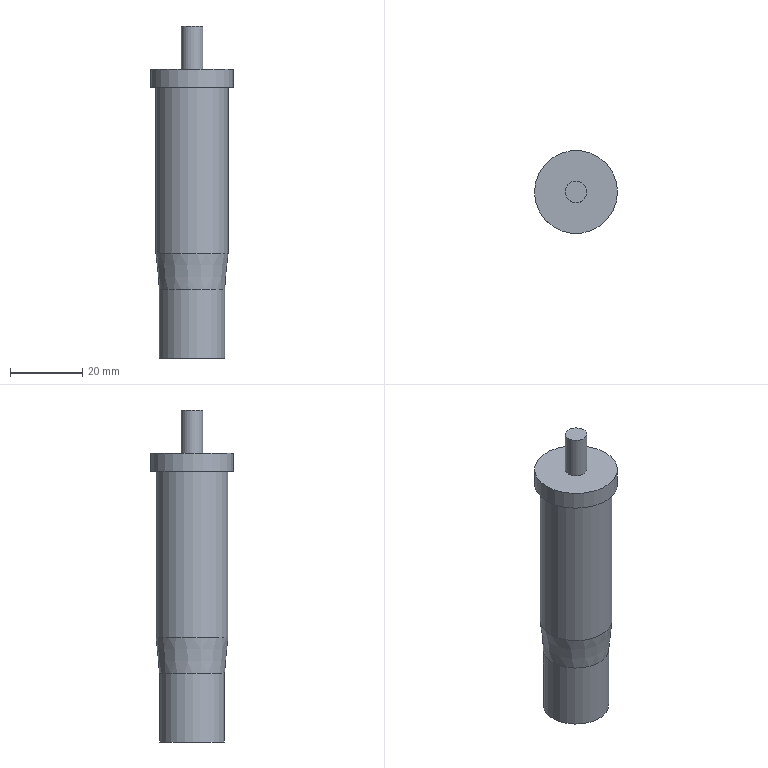Part | NX | features solid 2 | 1 solid | 9 faces | box 23 x 23 x 92 mm | volume 24609 mm3 | plane 4 | cylinder 4 | cone 1 | commonest cylinder face diameters 6 x1 18.1 x1 20 x1 23 x1
STEP:
#1=CARTESIAN_POINT('',(495.412,-159.012,39.));
#2=VERTEX_POINT('',#1);
#3=CARTESIAN_POINT('',(486.67,-161.354,39.));
#4=DIRECTION('',(0.,0.,1.));
#5=DIRECTION('',(0.9659,0.2588,0.));
#6=AXIS2_PLACEMENT_3D('',#3,#4,#5);
#7=CIRCLE('',#6,9.05);
#8=EDGE_CURVE('',#2,#2,#7,.T.);
#9=ORIENTED_EDGE('',*,*,#8,.F.);
#10=EDGE_LOOP('',(#9));
#11=FACE_BOUND('',#10,.T.);
#12=CARTESIAN_POINT('',(486.67,-161.354,39.));
#13=DIRECTION('',(0.,0.,-1.));
#14=DIRECTION('',(-0.9659,-0.2588,0.));
#15=AXIS2_PLACEMENT_3D('',#12,#13,#14);
#16=PLANE('',#15);
#17=ADVANCED_FACE('',(#11),#16,.T.);
#18=CARTESIAN_POINT('',(495.412,-159.012,58.));
#19=VERTEX_POINT('',#18);
#20=CARTESIAN_POINT('',(486.67,-161.354,58.));
#21=DIRECTION('',(0.,0.,1.));
#22=DIRECTION('',(0.9659,0.2588,0.));
#23=AXIS2_PLACEMENT_3D('',#20,#21,#22);
#24=CIRCLE('',#23,9.05);
#25=EDGE_CURVE('',#19,#19,#24,.T.);
#26=ORIENTED_EDGE('',*,*,#25,.F.);
#27=EDGE_LOOP('',(#26));
#28=FACE_BOUND('',#27,.T.);
#29=ORIENTED_EDGE('',*,*,#8,.T.);
#30=EDGE_LOOP('',(#29));
#31=FACE_BOUND('',#30,.T.);
#32=CARTESIAN_POINT('',(486.67,-161.354,39.));
#33=DIRECTION('',(0.,0.,1.));
#34=DIRECTION('',(0.9659,0.2588,0.));
#35=AXIS2_PLACEMENT_3D('',#32,#33,#34);
#36=CYLINDRICAL_SURFACE('',#35,9.05);
#37=ADVANCED_FACE('',(#28,#31),#36,.T.);
#38=ORIENTED_EDGE('',*,*,#25,.T.);
#39=EDGE_LOOP('',(#38));
#40=FACE_BOUND('',#39,.T.);
#41=CARTESIAN_POINT('',(496.329,-158.766,68.));
#42=VERTEX_POINT('',#41);
#43=CARTESIAN_POINT('',(486.67,-161.354,68.));
#44=DIRECTION('',(0.,0.,1.));
#45=DIRECTION('',(0.9659,0.2588,0.));
#46=AXIS2_PLACEMENT_3D('',#43,#44,#45);
#47=CIRCLE('',#46,10.);
#48=EDGE_CURVE('',#42,#42,#47,.T.);
#49=ORIENTED_EDGE('',*,*,#48,.F.);
#50=EDGE_LOOP('',(#49));
#51=FACE_BOUND('',#50,.T.);
#52=CARTESIAN_POINT('',(486.67,-161.354,58.));
#53=DIRECTION('',(0.,0.,1.));
#54=DIRECTION('',(0.9659,0.2588,0.));
#55=AXIS2_PLACEMENT_3D('',#52,#53,#54);
#56=CONICAL_SURFACE('',#55,9.05,0.09472);
#57=ADVANCED_FACE('',(#40,#51),#56,.T.);
#58=CARTESIAN_POINT('',(477.011,-163.943,114.));
#59=VERTEX_POINT('',#58);
#60=CARTESIAN_POINT('',(486.67,-161.354,114.));
#61=DIRECTION('',(0.,0.,-1.));
#62=DIRECTION('',(-0.9659,-0.2588,0.));
#63=AXIS2_PLACEMENT_3D('',#60,#61,#62);
#64=CIRCLE('',#63,10.);
#65=EDGE_CURVE('',#59,#59,#64,.F.);
#66=ORIENTED_EDGE('',*,*,#65,.F.);
#67=EDGE_LOOP('',(#66));
#68=FACE_BOUND('',#67,.T.);
#69=ORIENTED_EDGE('',*,*,#48,.T.);
#70=EDGE_LOOP('',(#69));
#71=FACE_BOUND('',#70,.T.);
#72=CARTESIAN_POINT('',(486.67,-161.354,68.));
#73=DIRECTION('',(0.,0.,1.));
#74=DIRECTION('',(0.9659,0.2588,0.));
#75=AXIS2_PLACEMENT_3D('',#72,#73,#74);
#76=CYLINDRICAL_SURFACE('',#75,10.);
#77=ADVANCED_FACE('',(#68,#71),#76,.T.);
#78=CARTESIAN_POINT('',(489.568,-160.578,119.));
#79=VERTEX_POINT('',#78);
#80=CARTESIAN_POINT('',(486.67,-161.354,119.));
#81=DIRECTION('',(0.,0.,1.));
#82=DIRECTION('',(0.9659,0.2588,0.));
#83=AXIS2_PLACEMENT_3D('',#80,#81,#82);
#84=CIRCLE('',#83,3.);
#85=EDGE_CURVE('',#79,#79,#84,.T.);
#86=ORIENTED_EDGE('',*,*,#85,.F.);
#87=EDGE_LOOP('',(#86));
#88=FACE_BOUND('',#87,.T.);
#89=CARTESIAN_POINT('',(475.562,-164.331,119.));
#90=VERTEX_POINT('',#89);
#91=CARTESIAN_POINT('',(486.67,-161.354,119.));
#92=DIRECTION('',(0.,0.,-1.));
#93=DIRECTION('',(-0.9659,-0.2588,0.));
#94=AXIS2_PLACEMENT_3D('',#91,#92,#93);
#95=CIRCLE('',#94,11.5);
#96=EDGE_CURVE('',#90,#90,#95,.T.);
#97=ORIENTED_EDGE('',*,*,#96,.F.);
#98=EDGE_LOOP('',(#97));
#99=FACE_BOUND('',#98,.T.);
#100=CARTESIAN_POINT('',(486.67,-161.354,119.));
#101=DIRECTION('',(0.,0.,1.));
#102=DIRECTION('',(0.9659,0.2588,0.));
#103=AXIS2_PLACEMENT_3D('',#100,#101,#102);
#104=PLANE('',#103);
#105=ADVANCED_FACE('',(#88,#99),#104,.T.);
#106=ORIENTED_EDGE('',*,*,#65,.T.);
#107=EDGE_LOOP('',(#106));
#108=FACE_BOUND('',#107,.T.);
#109=CARTESIAN_POINT('',(497.778,-158.378,114.));
#110=VERTEX_POINT('',#109);
#111=CARTESIAN_POINT('',(486.67,-161.354,114.));
#112=DIRECTION('',(0.,0.,1.));
#113=DIRECTION('',(0.9659,0.2588,0.));
#114=AXIS2_PLACEMENT_3D('',#111,#112,#113);
#115=CIRCLE('',#114,11.5);
#116=EDGE_CURVE('',#110,#110,#115,.T.);
#117=ORIENTED_EDGE('',*,*,#116,.F.);
#118=EDGE_LOOP('',(#117));
#119=FACE_BOUND('',#118,.T.);
#120=CARTESIAN_POINT('',(486.67,-161.354,114.));
#121=DIRECTION('',(0.,0.,-1.));
#122=DIRECTION('',(-0.9659,-0.2588,0.));
#123=AXIS2_PLACEMENT_3D('',#120,#121,#122);
#124=PLANE('',#123);
#125=ADVANCED_FACE('',(#108,#119),#124,.T.);
#126=ORIENTED_EDGE('',*,*,#96,.T.);
#127=EDGE_LOOP('',(#126));
#128=FACE_BOUND('',#127,.T.);
#129=ORIENTED_EDGE('',*,*,#116,.T.);
#130=EDGE_LOOP('',(#129));
#131=FACE_BOUND('',#130,.T.);
#132=CARTESIAN_POINT('',(486.67,-161.354,114.));
#133=DIRECTION('',(0.,0.,1.));
#134=DIRECTION('',(0.9659,0.2588,0.));
#135=AXIS2_PLACEMENT_3D('',#132,#133,#134);
#136=CYLINDRICAL_SURFACE('',#135,11.5);
#137=ADVANCED_FACE('',(#128,#131),#136,.T.);
#138=CARTESIAN_POINT('',(483.772,-162.131,131.));
#139=VERTEX_POINT('',#138);
#140=CARTESIAN_POINT('',(486.67,-161.354,131.));
#141=DIRECTION('',(0.,0.,-1.));
#142=DIRECTION('',(-0.9659,-0.2588,0.));
#143=AXIS2_PLACEMENT_3D('',#140,#141,#142);
#144=CIRCLE('',#143,3.);
#145=EDGE_CURVE('',#139,#139,#144,.T.);
#146=ORIENTED_EDGE('',*,*,#145,.F.);
#147=EDGE_LOOP('',(#146));
#148=FACE_BOUND('',#147,.T.);
#149=CARTESIAN_POINT('',(486.67,-161.354,131.));
#150=DIRECTION('',(0.,0.,1.));
#151=DIRECTION('',(0.9659,0.2588,0.));
#152=AXIS2_PLACEMENT_3D('',#149,#150,#151);
#153=PLANE('',#152);
#154=ADVANCED_FACE('',(#148),#153,.T.);
#155=ORIENTED_EDGE('',*,*,#145,.T.);
#156=EDGE_LOOP('',(#155));
#157=FACE_BOUND('',#156,.T.);
#158=ORIENTED_EDGE('',*,*,#85,.T.);
#159=EDGE_LOOP('',(#158));
#160=FACE_BOUND('',#159,.T.);
#161=CARTESIAN_POINT('',(486.67,-161.354,119.));
#162=DIRECTION('',(0.,0.,1.));
#163=DIRECTION('',(0.9659,0.2588,0.));
#164=AXIS2_PLACEMENT_3D('',#161,#162,#163);
#165=CYLINDRICAL_SURFACE('',#164,3.);
#166=ADVANCED_FACE('',(#157,#160),#165,.T.);
#167=CLOSED_SHELL('',(#17,#37,#57,#77,#105,#125,#137,#154,#166));
#168=MANIFOLD_SOLID_BREP('',#167);
#169=(LENGTH_UNIT()NAMED_UNIT(*)SI_UNIT(.MILLI.,.METRE.));
#170=UNCERTAINTY_MEASURE_WITH_UNIT(LENGTH_MEASURE(0.00001),#169,'','');
#171=(NAMED_UNIT(*)PLANE_ANGLE_UNIT()SI_UNIT($,.RADIAN.));
#172=(NAMED_UNIT(*)SI_UNIT($,.STERADIAN.)SOLID_ANGLE_UNIT());
#173=(GEOMETRIC_REPRESENTATION_CONTEXT(3)GLOBAL_UNCERTAINTY_ASSIGNED_CONTEXT((#170))GLOBAL_UNIT_ASSIGNED_CONTEXT((#169,#171,#172))REPRESENTATION_CONTEXT('',''));
#174=ADVANCED_BREP_SHAPE_REPRESENTATION('',(#168),#173);